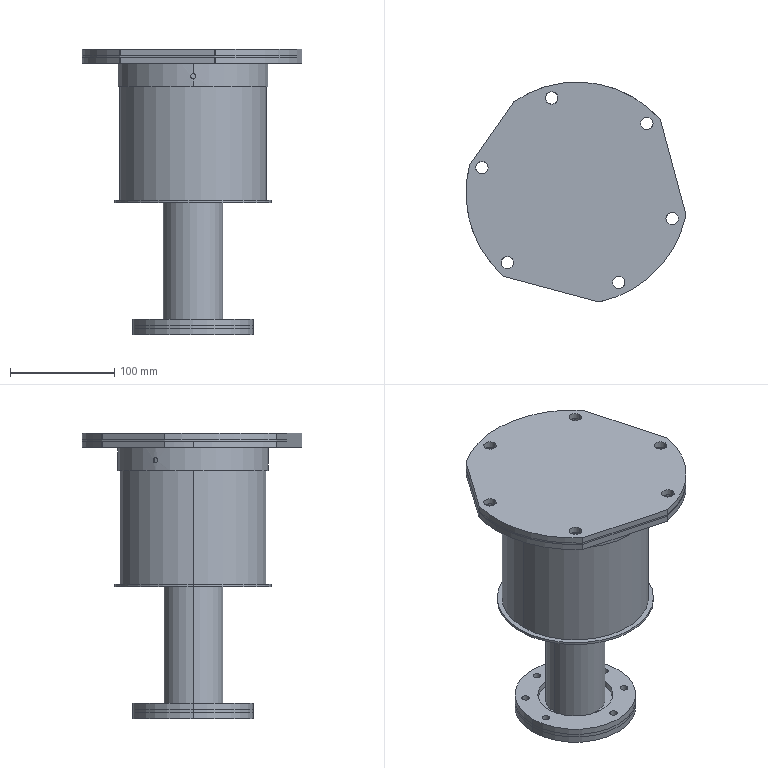Part | SolidWorks | features CompositeCurve 1 | 9 solids | 172 faces | box 210.92 x 210.92 x 274.1 mm | volume 648212 mm3 | cylinder 138 | plane 30 | torus 4 | commonest cylinder face diameters 7.2 x36 12 x36 2 x19 213 x11 5 x6 116 x6